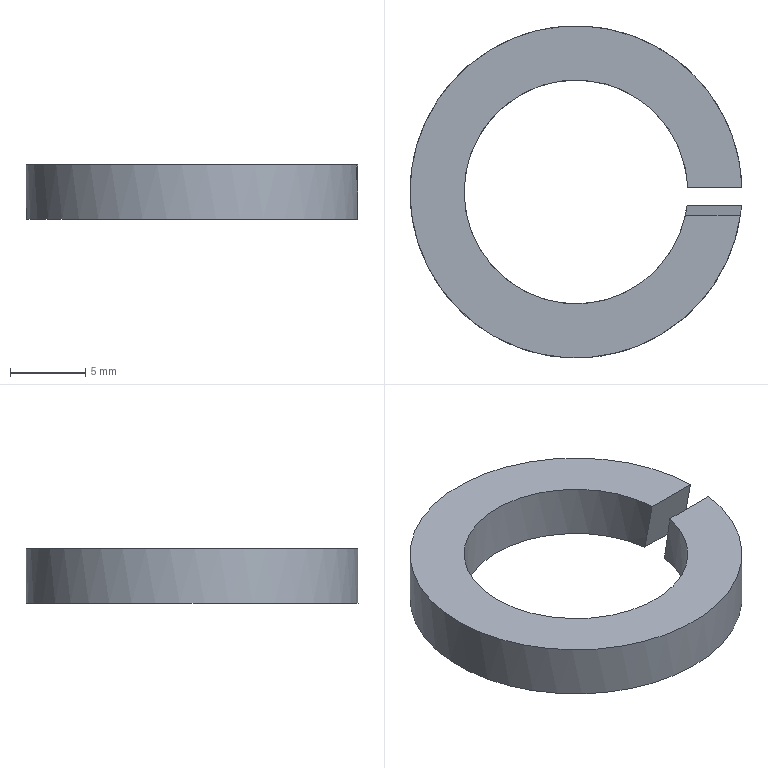Part | NX | 1 solid | 6 faces | box 22.096 x 22.1 x 3.6 mm | volume 729.48 mm3 | plane 4 | cylinder 2 | commonest cylinder face diameters 14.9 x1 22.1 x1
STEP:
#1=CARTESIAN_POINT('',(11.012,-0.9139,0.));
#2=VERTEX_POINT('',#1);
#3=CARTESIAN_POINT('',(11.012,0.9139,0.));
#4=VERTEX_POINT('',#3);
#5=CARTESIAN_POINT('',(0.,0.,0.));
#6=DIRECTION('',(0.,0.,-1.));
#7=DIRECTION('',(-1.,0.,0.));
#8=AXIS2_PLACEMENT_3D('',#5,#6,#7);
#9=CIRCLE('',#8,11.05);
#10=EDGE_CURVE('',#2,#4,#9,.T.);
#11=ORIENTED_EDGE('',*,*,#10,.F.);
#12=CARTESIAN_POINT('',(10.941,-1.549,3.6));
#13=VERTEX_POINT('',#12);
#14=CARTESIAN_POINT('',(0.,0.,-5.183));
#15=DIRECTION('',(0.,-0.9848,-0.1736));
#16=DIRECTION('',(0.,0.1736,-0.9848));
#17=AXIS2_PLACEMENT_3D('',#14,#15,#16);
#18=ELLIPSE('',#17,63.634,11.05);
#19=EDGE_CURVE('',#2,#13,#18,.T.);
#20=ORIENTED_EDGE('',*,*,#19,.T.);
#21=CARTESIAN_POINT('',(11.046,0.2791,3.6));
#22=VERTEX_POINT('',#21);
#23=CARTESIAN_POINT('',(0.,0.,3.6));
#24=DIRECTION('',(0.,0.,-1.));
#25=DIRECTION('',(-1.,0.,0.));
#26=AXIS2_PLACEMENT_3D('',#23,#24,#25);
#27=CIRCLE('',#26,11.05);
#28=EDGE_CURVE('',#13,#22,#27,.T.);
#29=ORIENTED_EDGE('',*,*,#28,.T.);
#30=CARTESIAN_POINT('',(0.,0.,5.183));
#31=DIRECTION('',(0.,0.9848,0.1736));
#32=DIRECTION('',(0.,0.1736,-0.9848));
#33=AXIS2_PLACEMENT_3D('',#30,#31,#32);
#34=ELLIPSE('',#33,63.634,11.05);
#35=EDGE_CURVE('',#22,#4,#34,.T.);
#36=ORIENTED_EDGE('',*,*,#35,.T.);
#37=EDGE_LOOP('',(#11,#20,#29,#36));
#38=FACE_OUTER_BOUND('',#37,.T.);
#39=CARTESIAN_POINT('',(0.,0.,0.));
#40=DIRECTION('',(0.,0.,-1.));
#41=DIRECTION('',(1.,0.,0.));
#42=AXIS2_PLACEMENT_3D('',#39,#40,#41);
#43=CYLINDRICAL_SURFACE('',#42,11.05);
#44=ADVANCED_FACE('',(#38),#43,.T.);
#45=ORIENTED_EDGE('',*,*,#28,.F.);
#46=CARTESIAN_POINT('',(7.287,-1.549,3.6));
#47=VERTEX_POINT('',#46);
#48=CARTESIAN_POINT('',(0.,-1.549,3.6));
#49=DIRECTION('',(-1.,0.,0.));
#50=VECTOR('',#49,1.);
#51=LINE('',#48,#50);
#52=EDGE_CURVE('',#13,#47,#51,.T.);
#53=ORIENTED_EDGE('',*,*,#52,.T.);
#54=CARTESIAN_POINT('',(7.445,0.2791,3.6));
#55=VERTEX_POINT('',#54);
#56=CARTESIAN_POINT('',(0.,0.,3.6));
#57=DIRECTION('',(0.,0.,-1.));
#58=DIRECTION('',(-1.,0.,0.));
#59=AXIS2_PLACEMENT_3D('',#56,#57,#58);
#60=CIRCLE('',#59,7.45);
#61=EDGE_CURVE('',#47,#55,#60,.T.);
#62=ORIENTED_EDGE('',*,*,#61,.T.);
#63=CARTESIAN_POINT('',(0.,0.2791,3.6));
#64=DIRECTION('',(1.,0.,0.));
#65=VECTOR('',#64,1.);
#66=LINE('',#63,#65);
#67=EDGE_CURVE('',#55,#22,#66,.T.);
#68=ORIENTED_EDGE('',*,*,#67,.T.);
#69=EDGE_LOOP('',(#45,#53,#62,#68));
#70=FACE_OUTER_BOUND('',#69,.T.);
#71=CARTESIAN_POINT('',(0.,11.05,3.6));
#72=DIRECTION('',(0.,0.,1.));
#73=DIRECTION('',(-1.,0.,0.));
#74=AXIS2_PLACEMENT_3D('',#71,#72,#73);
#75=PLANE('',#74);
#76=ADVANCED_FACE('',(#70),#75,.T.);
#77=ORIENTED_EDGE('',*,*,#61,.F.);
#78=CARTESIAN_POINT('',(7.394,-0.9139,0.));
#79=VERTEX_POINT('',#78);
#80=CARTESIAN_POINT('',(0.,0.,-5.183));
#81=DIRECTION('',(0.,0.9848,0.1736));
#82=DIRECTION('',(0.,0.1736,-0.9848));
#83=AXIS2_PLACEMENT_3D('',#80,#81,#82);
#84=ELLIPSE('',#83,42.903,7.45);
#85=EDGE_CURVE('',#47,#79,#84,.T.);
#86=ORIENTED_EDGE('',*,*,#85,.T.);
#87=CARTESIAN_POINT('',(7.394,0.9139,0.));
#88=VERTEX_POINT('',#87);
#89=CARTESIAN_POINT('',(0.,0.,0.));
#90=DIRECTION('',(0.,0.,-1.));
#91=DIRECTION('',(-1.,0.,0.));
#92=AXIS2_PLACEMENT_3D('',#89,#90,#91);
#93=CIRCLE('',#92,7.45);
#94=EDGE_CURVE('',#79,#88,#93,.T.);
#95=ORIENTED_EDGE('',*,*,#94,.T.);
#96=CARTESIAN_POINT('',(0.,0.,5.183));
#97=DIRECTION('',(0.,-0.9848,-0.1736));
#98=DIRECTION('',(0.,0.1736,-0.9848));
#99=AXIS2_PLACEMENT_3D('',#96,#97,#98);
#100=ELLIPSE('',#99,42.903,7.45);
#101=EDGE_CURVE('',#88,#55,#100,.T.);
#102=ORIENTED_EDGE('',*,*,#101,.T.);
#103=EDGE_LOOP('',(#77,#86,#95,#102));
#104=FACE_OUTER_BOUND('',#103,.T.);
#105=CARTESIAN_POINT('',(0.,0.,0.));
#106=DIRECTION('',(0.,0.,-1.));
#107=DIRECTION('',(1.,0.,0.));
#108=AXIS2_PLACEMENT_3D('',#105,#106,#107);
#109=CYLINDRICAL_SURFACE('',#108,7.45);
#110=ADVANCED_FACE('',(#104),#109,.F.);
#111=ORIENTED_EDGE('',*,*,#94,.F.);
#112=CARTESIAN_POINT('',(0.,-0.9139,0.));
#113=DIRECTION('',(1.,0.,0.));
#114=VECTOR('',#113,1.);
#115=LINE('',#112,#114);
#116=EDGE_CURVE('',#79,#2,#115,.T.);
#117=ORIENTED_EDGE('',*,*,#116,.T.);
#118=ORIENTED_EDGE('',*,*,#10,.T.);
#119=CARTESIAN_POINT('',(0.,0.9139,0.));
#120=DIRECTION('',(-1.,0.,0.));
#121=VECTOR('',#120,1.);
#122=LINE('',#119,#121);
#123=EDGE_CURVE('',#4,#88,#122,.T.);
#124=ORIENTED_EDGE('',*,*,#123,.T.);
#125=EDGE_LOOP('',(#111,#117,#118,#124));
#126=FACE_OUTER_BOUND('',#125,.T.);
#127=CARTESIAN_POINT('',(0.,7.45,0.));
#128=DIRECTION('',(0.,0.,-1.));
#129=DIRECTION('',(1.,0.,0.));
#130=AXIS2_PLACEMENT_3D('',#127,#128,#129);
#131=PLANE('',#130);
#132=ADVANCED_FACE('',(#126),#131,.T.);
#133=ORIENTED_EDGE('',*,*,#67,.F.);
#134=ORIENTED_EDGE('',*,*,#101,.F.);
#135=ORIENTED_EDGE('',*,*,#123,.F.);
#136=ORIENTED_EDGE('',*,*,#35,.F.);
#137=EDGE_LOOP('',(#133,#134,#135,#136));
#138=FACE_OUTER_BOUND('',#137,.T.);
#139=CARTESIAN_POINT('',(16.575,1.824,-5.162));
#140=DIRECTION('',(0.,-0.9848,-0.1736));
#141=DIRECTION('',(0.,-0.1736,0.9848));
#142=AXIS2_PLACEMENT_3D('',#139,#140,#141);
#143=PLANE('',#142);
#144=ADVANCED_FACE('',(#138),#143,.T.);
#145=ORIENTED_EDGE('',*,*,#116,.F.);
#146=ORIENTED_EDGE('',*,*,#85,.F.);
#147=ORIENTED_EDGE('',*,*,#52,.F.);
#148=ORIENTED_EDGE('',*,*,#19,.F.);
#149=EDGE_LOOP('',(#145,#146,#147,#148));
#150=FACE_OUTER_BOUND('',#149,.T.);
#151=CARTESIAN_POINT('',(16.575,-1.824,5.162));
#152=DIRECTION('',(0.,0.9848,0.1736));
#153=DIRECTION('',(0.,0.1736,-0.9848));
#154=AXIS2_PLACEMENT_3D('',#151,#152,#153);
#155=PLANE('',#154);
#156=ADVANCED_FACE('',(#150),#155,.T.);
#157=CLOSED_SHELL('',(#44,#76,#110,#132,#144,#156));
#158=MANIFOLD_SOLID_BREP('',#157);
#159=(LENGTH_UNIT()NAMED_UNIT(*)SI_UNIT(.MILLI.,.METRE.));
#160=UNCERTAINTY_MEASURE_WITH_UNIT(LENGTH_MEASURE(0.00002),#159,'','');
#161=(NAMED_UNIT(*)PLANE_ANGLE_UNIT()SI_UNIT($,.RADIAN.));
#162=PLANE_ANGLE_MEASURE_WITH_UNIT(PLANE_ANGLE_MEASURE(0.01745),#161);
#163=DIMENSIONAL_EXPONENTS(0.,0.,0.,0.,0.,0.,0.);
#164=(CONVERSION_BASED_UNIT('DEGREE',#162)NAMED_UNIT(#163)PLANE_ANGLE_UNIT());
#165=(NAMED_UNIT(*)SI_UNIT($,.STERADIAN.)SOLID_ANGLE_UNIT());
#166=(GEOMETRIC_REPRESENTATION_CONTEXT(3)GLOBAL_UNCERTAINTY_ASSIGNED_CONTEXT((#160))GLOBAL_UNIT_ASSIGNED_CONTEXT((#159,#164,#165))REPRESENTATION_CONTEXT('',''));
#167=ADVANCED_BREP_SHAPE_REPRESENTATION('',(#158),#166);